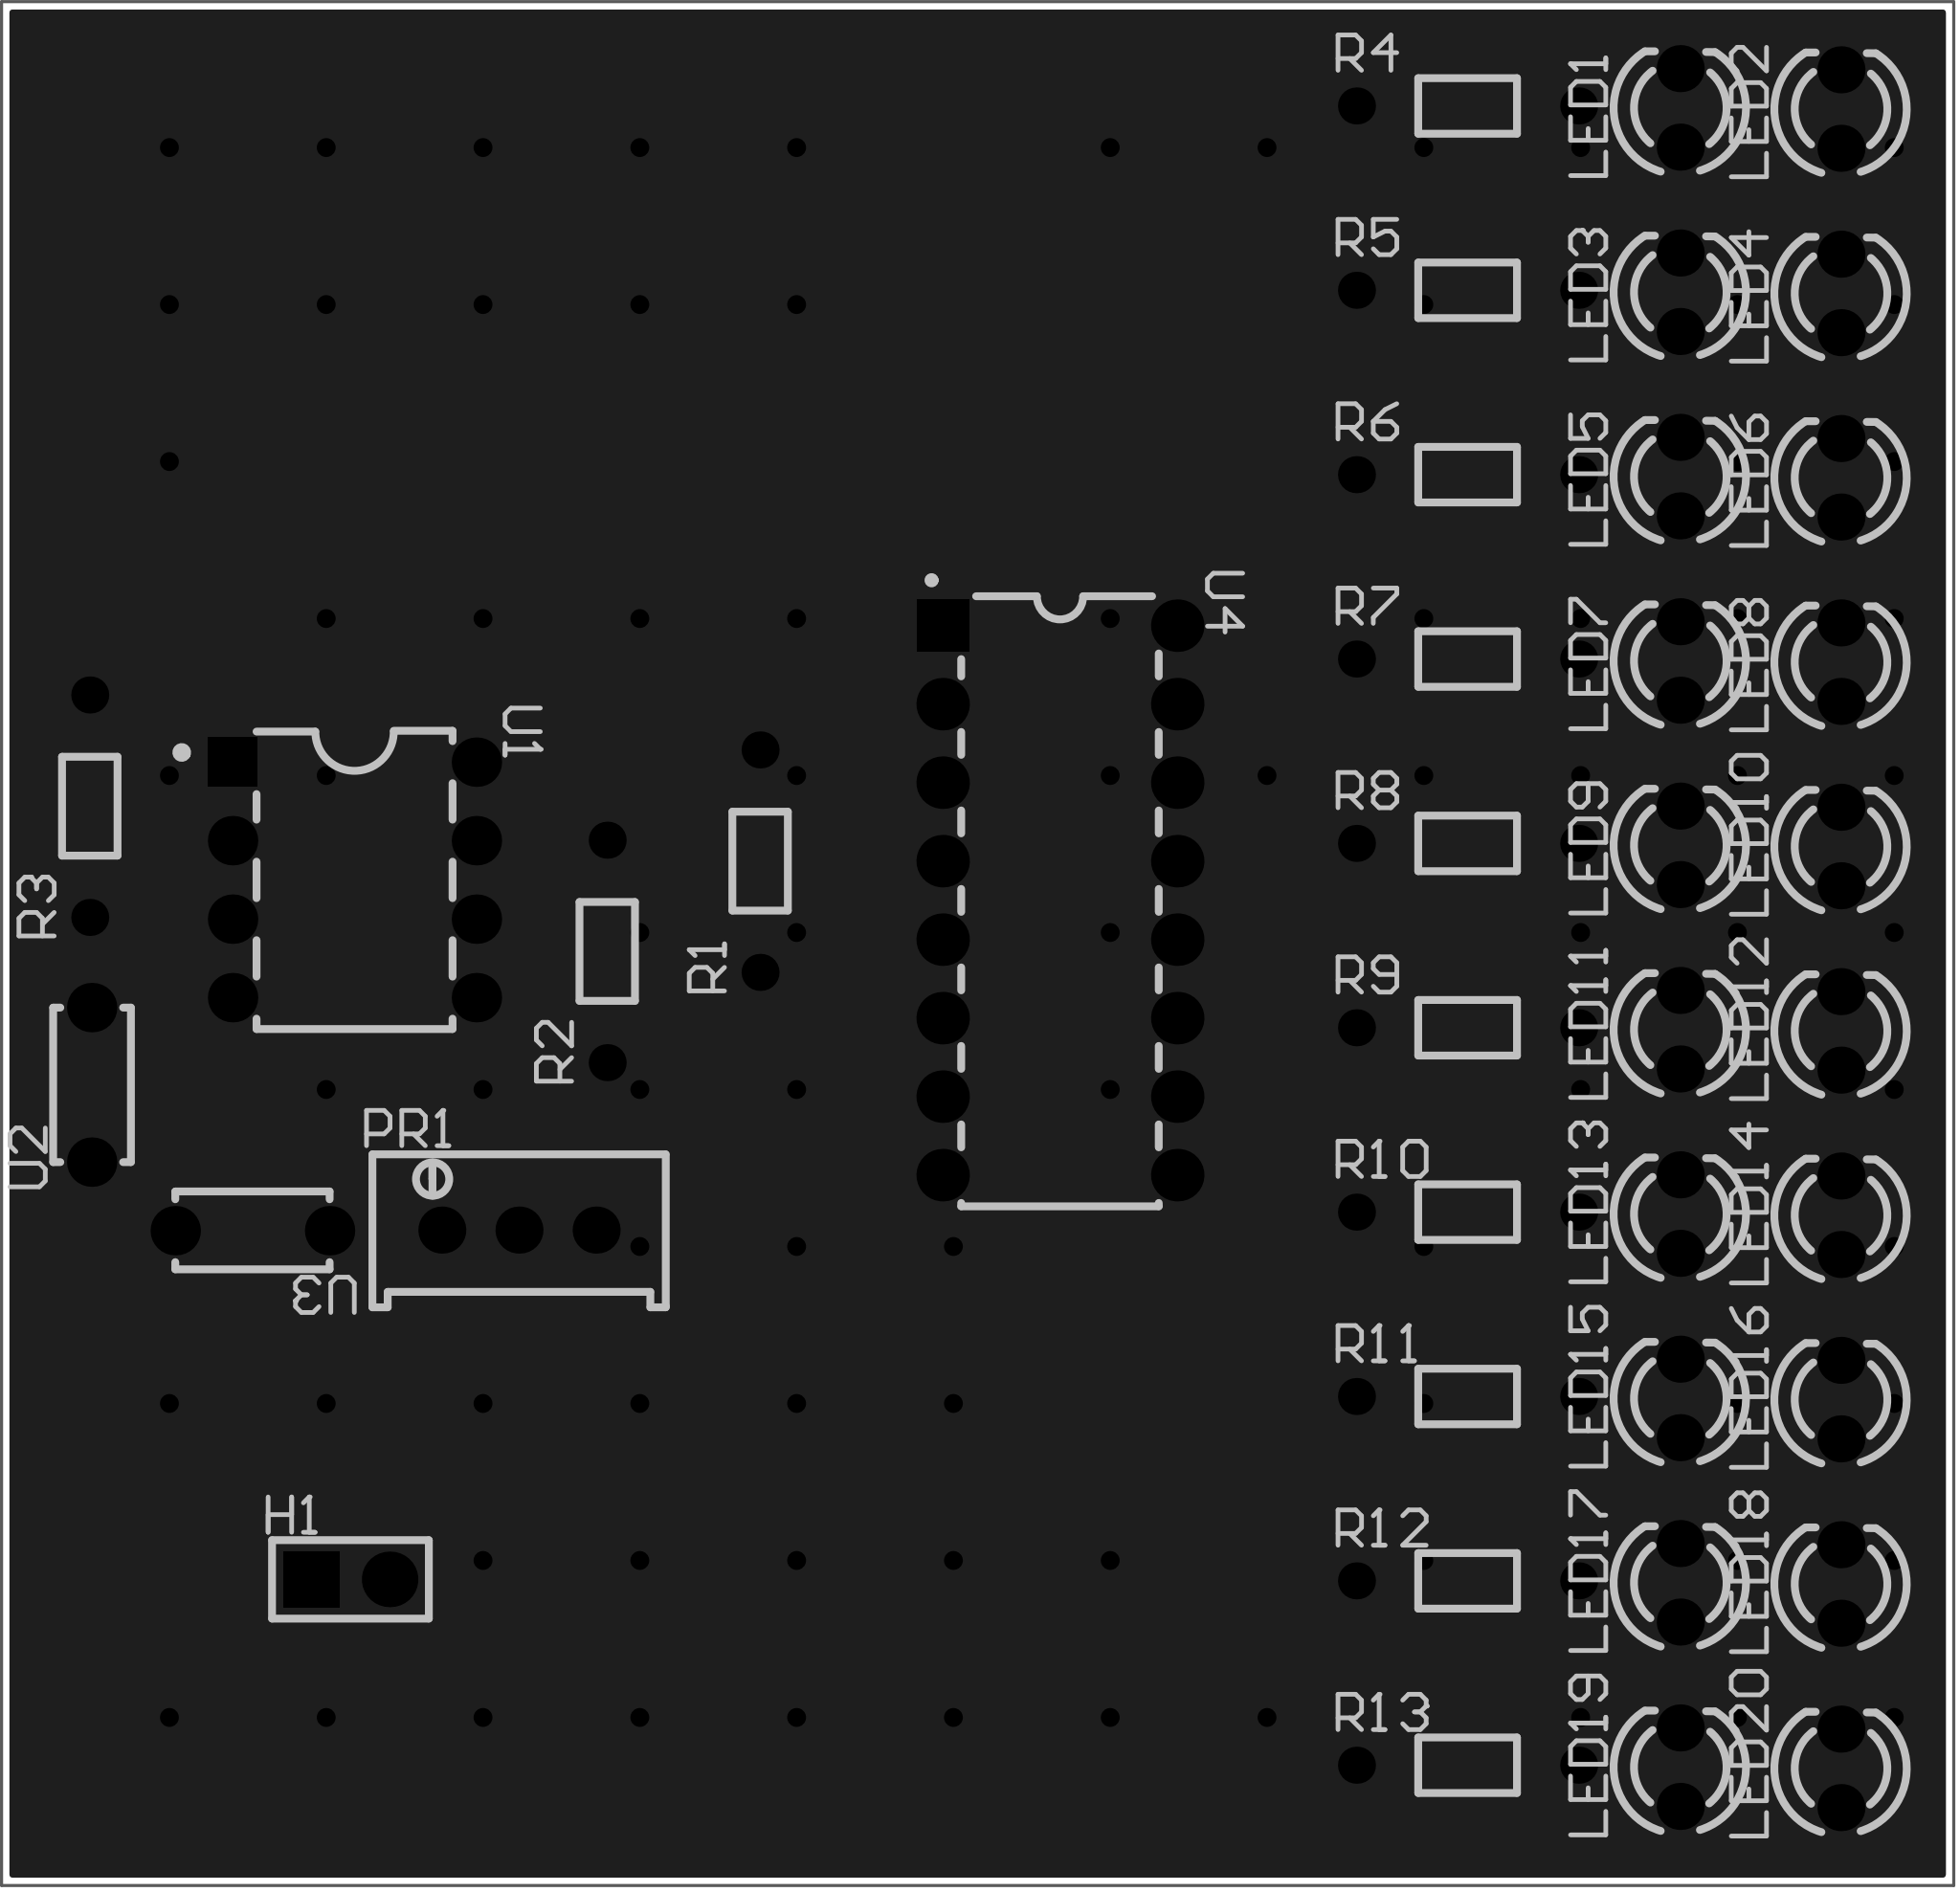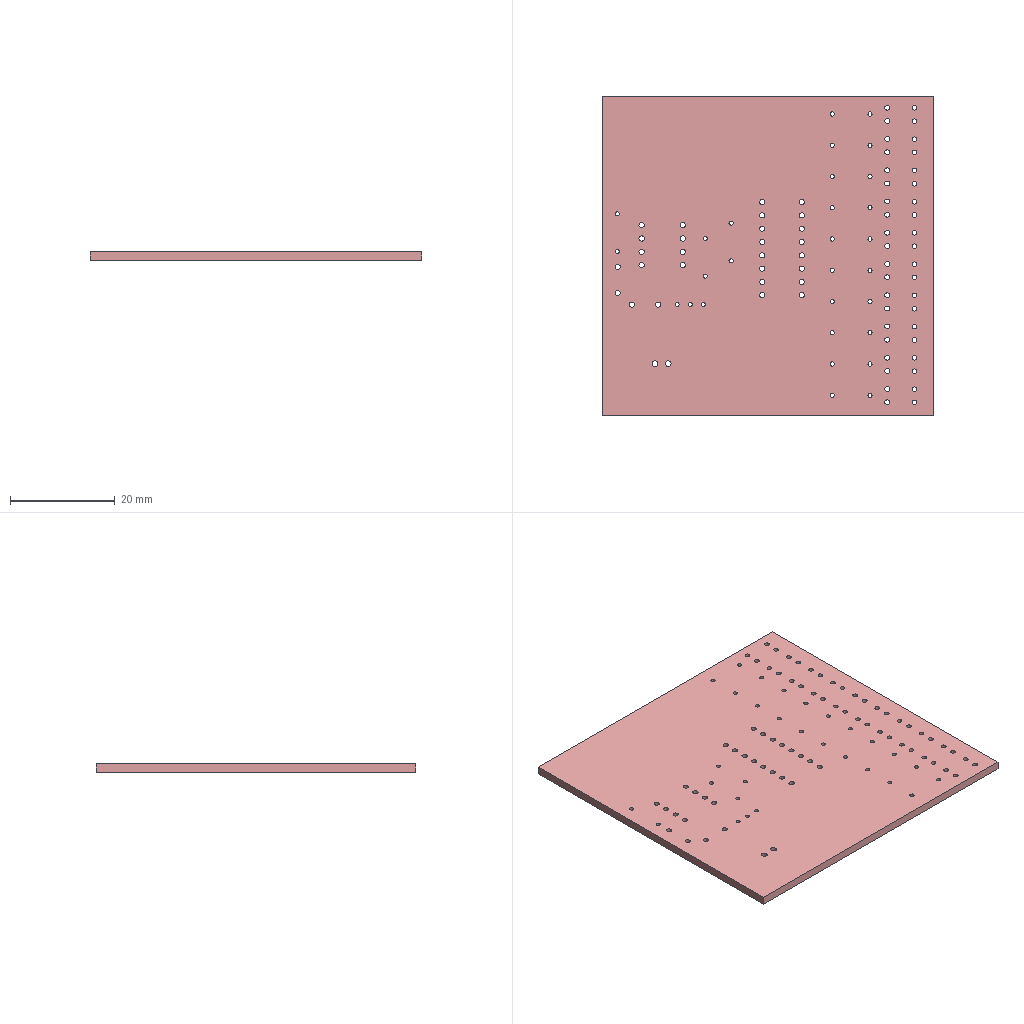Circuit board layout | Altium Designer | box 63.2 x 61 x 1.6 mm
Layer stack:
# Altium Designer layer stack of  (unit mm; dielectric type: 0 none, 1 core, 2 prepreg, 3 surface material)
index,name,kind,layer,copper_thickness_mm,dielectric_type,dielectric_thickness_mm,dielectric_material,dielectric_constant
0,Top Paste Mask Layer,other,,,,,,
1,Top Silkscreen Layer,other,,,,,,
2,Top Solder Mask Layer,dielectric,,,3,0.01,,3.3
3,Top Layer,copper,Top Layer,0.035,,,,
4,Dielectric1,dielectric,,,3,1.51,FR4,4.5
5,Bottom Layer,copper,Bottom Layer,0.035,,,,
6,Bottom Solder Mask Layer,dielectric,,,3,0.01,,3.3
7,Bottom Silkscreen Layer,other,,,,,,
8,Bottom Paste Mask Layer,other,,,,,,
# drill layer pairs: low layer,high layer
drill_pair,Top Layer,Bottom Layer
Part placement:
Designator,Comment,Layer,Footprint,Center-X(mm),Center-Y(mm),Rotation
H1,,TopLayer,HDR-TH_2P-P2.54-V-M-1,100.33,91.567,0
LED1,,TopLayer,LED_TH-3mm,143.413,139.183,90
LED2,,TopLayer,LED_TH-3mm,148.62,139.145,90
LED3,,TopLayer,LED_TH-3mm,143.413,133.217,90
LED4,,TopLayer,LED_TH-3mm,148.62,133.179,90
LED5,,TopLayer,LED_TH-3mm,143.413,127.251,90
LED6,,TopLayer,LED_TH-3mm,148.62,127.213,90
LED7,,TopLayer,LED_TH-3mm,143.413,121.285,90
LED8,,TopLayer,LED_TH-3mm,148.62,121.247,90
LED9,,TopLayer,LED_TH-3mm,143.413,115.32,90
LED10,,TopLayer,LED_TH-3mm,148.62,115.282,90
LED11,,TopLayer,LED_TH-3mm,143.413,109.354,90
LED12,,TopLayer,LED_TH-3mm,148.62,109.316,90
LED13,,TopLayer,LED_TH-3mm,143.413,103.388,90
LED14,,TopLayer,LED_TH-3mm,148.62,103.35,90
LED15,,TopLayer,LED_TH-3mm,143.413,97.422,90
LED16,,TopLayer,LED_TH-3mm,148.62,97.384,90
LED17,,TopLayer,LED_TH-3mm,143.413,91.456,90
LED18,,TopLayer,LED_TH-3mm,148.62,91.418,90
LED19,,TopLayer,LED_TH-3mm,143.413,85.49,90
LED20,,TopLayer,LED_TH-3mm,148.62,85.452,90
PR1,10kΩ,TopLayer,R_3296,105.791,102.87,0
R1,2.2kΩ,TopLayer,Res_1/8W,113.602,114.808,90
R2,10kΩ,TopLayer,Res_1/8W,108.649,111.887,90
R3,10kΩ,TopLayer,Res_1/8W,91.885,116.586,90
R4,10Ω,TopLayer,Res_1/8W,136.523,139.246,0
R5,10Ω,TopLayer,Res_1/8W,136.523,133.28,0
R6,10Ω,TopLayer,Res_1/8W,136.523,127.314,0
R7,10Ω,TopLayer,Res_1/8W,136.523,121.348,0
R8,10Ω,TopLayer,Res_1/8W,136.523,115.383,0
R9,10Ω,TopLayer,Res_1/8W,136.523,109.417,0
R10,10Ω,TopLayer,Res_1/8W,136.523,103.451,0
R11,10Ω,TopLayer,Res_1/8W,136.523,97.485,0
R12,10Ω,TopLayer,Res_1/8W,136.523,91.519,0
R13,10Ω,TopLayer,Res_1/8W,136.523,85.553,0
U1,NE555PE4,TopLayer,PDIP-8_L9.6-W6.4-P2.54-LS7.9-BL-1,100.462,114.201,270
U2,100nF,TopLayer,CAP-TH_L5.0-W2.5-P5.00-D1.0,91.948,107.569,90
U3,1uF,TopLayer,CAP-TH_L5.0-W2.5-P5.00-D1.0,97.155,102.85,180
U4,4017BDM,TopLayer,PDIP-16_L19.3-W6.5-P2.54-LS7.6-BL,123.317,113.538,270
Pad and via stacks:
# Altium Designer via and pad stacks of  (unit mm). Each distinct definition once, with the count of objects using it.
# via: kind,start_layer,end_layer,hole_mm,diameter_mm,mode(0 simple;1 top-mid-bottom;2 full stack),diameter_per_layer,count,example_net
# pad: kind,layer,hole_mm,hole_type(0 round;1 square;2 slot),plating,top_size,top_shape(1 round;2 rect;3 octagon;9 rounded rect),mid_size,bottom_size,mode,footprint,size_per_layer,count,example
pad,Multi-Layer,1.1,0,plated,1.8x1.8,1,1.8x1.8,1.8x1.8,0,HDR-TH_2P-P2.54-V-M-1,,1,H1.2
pad,Multi-Layer,1.1,0,plated,1.8x1.8,2,1.8x1.8,1.8x1.8,0,HDR-TH_2P-P2.54-V-M-1,,1,H1.1
pad,Multi-Layer,0.9144,0,plated,1.524x1.524,1,1.524x1.524,1.524x1.524,0,LED_TH-3mm,,40,LED1.1
pad,Multi-Layer,0.762,0,plated,1.524x1.524,1,1.524x1.524,1.524x1.524,0,R_3296,,3,PR1.2
pad,Multi-Layer,0.8001,0,plated,1.199x1.199,1,1.199x1.199,1.199x1.199,0,Res_1/8W,,26,R1.1
pad,Multi-Layer,1,0,plated,1.6x1.6,1,1.6x1.6,1.6x1.6,0,PDIP-8_L9.6-W6.4-P2.54-LS7.9-BL-1,,7,U1.8
pad,Multi-Layer,1,0,plated,1.6x1.6,2,1.6x1.6,1.6x1.6,0,PDIP-8_L9.6-W6.4-P2.54-LS7.9-BL-1,,1,U1.1
pad,Multi-Layer,1,0,plated,1.6x1.6,1,1.6x1.6,1.6x1.6,0,CAP-TH_L5.0-W2.5-P5.00-D1.0,,4,U2.1
pad,Multi-Layer,1,0,plated,1.7x1.7,2,1.7x1.7,1.7x1.7,0,PDIP-16_L19.3-W6.5-P2.54-LS7.6-BL,,1,U4.1
pad,Multi-Layer,1,0,plated,1.7x1.7,1,1.7x1.7,1.7x1.7,0,PDIP-16_L19.3-W6.5-P2.54-LS7.6-BL,,15,U4.2
via,Top Layer,Bottom Layer,0.3048,0.61,0,,85,GND
Copper pours:
name,layer,net,type(0 solid;1 hatched;2 none)
Top Layer-GND,Top Layer,GND,0
Bottom Layer-GND,Bottom Layer,GND,0
Design rules, without the lines most boards share:
# Altium Designer design rules of  (exported by Altium Designer, unit mm)
# columns: name | kind | enabled | priority | scope1 | scope2 | descriptor | typed fields (field=value)
creepage | 65 | enabled | 1 | All | All | Creepage Distance Constraint =(0mil) (All),(All) |